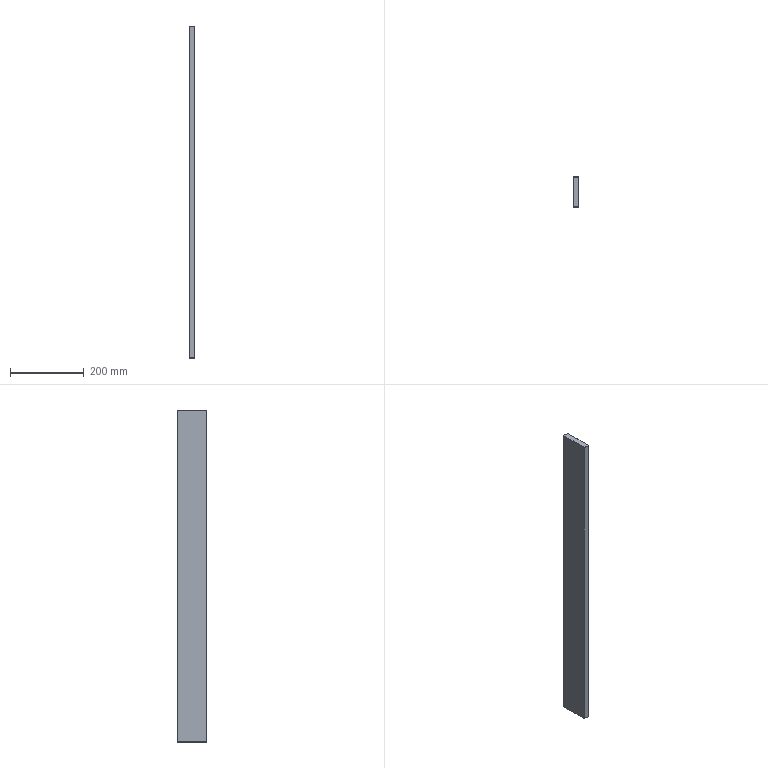Part | STEP file | HJDX-007 | 1 solid | 26 faces | box 16 x 80 x 900 mm | volume 1151503 mm3 | plane 26
STEP:
#1=CARTESIAN_POINT('',(16.,-39.5,-449.5));
#2=VERTEX_POINT('',#1);
#3=CARTESIAN_POINT('',(16.,-39.5,449.5));
#4=VERTEX_POINT('',#3);
#5=CARTESIAN_POINT('',(16.,-39.5,0.));
#6=DIRECTION('',(0.,0.,1.));
#7=VECTOR('',#6,1000.);
#8=LINE('',#5,#7);
#9=EDGE_CURVE('',#2,#4,#8,.T.);
#10=ORIENTED_EDGE('',*,*,#9,.F.);
#11=CARTESIAN_POINT('',(16.,39.5,-449.5));
#12=VERTEX_POINT('',#11);
#13=CARTESIAN_POINT('',(16.,0.,-449.5));
#14=DIRECTION('',(0.,-1.,0.));
#15=VECTOR('',#14,1000.);
#16=LINE('',#13,#15);
#17=EDGE_CURVE('',#12,#2,#16,.T.);
#18=ORIENTED_EDGE('',*,*,#17,.F.);
#19=CARTESIAN_POINT('',(16.,39.5,449.5));
#20=VERTEX_POINT('',#19);
#21=CARTESIAN_POINT('',(16.,39.5,0.));
#22=DIRECTION('',(0.,0.,-1.));
#23=VECTOR('',#22,1000.);
#24=LINE('',#21,#23);
#25=EDGE_CURVE('',#20,#12,#24,.T.);
#26=ORIENTED_EDGE('',*,*,#25,.F.);
#27=CARTESIAN_POINT('',(16.,0.,449.5));
#28=DIRECTION('',(0.,1.,0.));
#29=VECTOR('',#28,1000.);
#30=LINE('',#27,#29);
#31=EDGE_CURVE('',#4,#20,#30,.T.);
#32=ORIENTED_EDGE('',*,*,#31,.F.);
#33=EDGE_LOOP('',(#10,#18,#26,#32));
#34=FACE_OUTER_BOUND('',#33,.T.);
#35=CARTESIAN_POINT('',(16.,0.,0.));
#36=DIRECTION('',(-1.,0.,0.));
#37=DIRECTION('',(0.,0.,1.));
#38=AXIS2_PLACEMENT_3D('',#35,#36,#37);
#39=PLANE('',#38);
#40=ADVANCED_FACE('',(#34),#39,.F.);
#41=ORIENTED_EDGE('',*,*,#31,.T.);
#42=CARTESIAN_POINT('',(15.5,39.5,450.));
#43=VERTEX_POINT('',#42);
#44=CARTESIAN_POINT('',(16.,39.5,449.5));
#45=DIRECTION('',(0.7071,0.,-0.7071));
#46=VECTOR('',#45,1000.);
#47=LINE('',#44,#46);
#48=EDGE_CURVE('',#43,#20,#47,.T.);
#49=ORIENTED_EDGE('',*,*,#48,.F.);
#50=CARTESIAN_POINT('',(15.5,-39.5,450.));
#51=VERTEX_POINT('',#50);
#52=CARTESIAN_POINT('',(15.5,0.,450.));
#53=DIRECTION('',(0.,1.,0.));
#54=VECTOR('',#53,1000.);
#55=LINE('',#52,#54);
#56=EDGE_CURVE('',#51,#43,#55,.T.);
#57=ORIENTED_EDGE('',*,*,#56,.F.);
#58=CARTESIAN_POINT('',(16.,-39.5,449.5));
#59=DIRECTION('',(-0.7071,0.,0.7071));
#60=VECTOR('',#59,1000.);
#61=LINE('',#58,#60);
#62=EDGE_CURVE('',#4,#51,#61,.T.);
#63=ORIENTED_EDGE('',*,*,#62,.F.);
#64=EDGE_LOOP('',(#41,#49,#57,#63));
#65=FACE_OUTER_BOUND('',#64,.T.);
#66=CARTESIAN_POINT('',(16.,0.,449.5));
#67=DIRECTION('',(-0.7071,0.,-0.7071));
#68=DIRECTION('',(-0.7071,0.,0.7071));
#69=AXIS2_PLACEMENT_3D('',#66,#67,#68);
#70=PLANE('',#69);
#71=ADVANCED_FACE('',(#65),#70,.F.);
#72=ORIENTED_EDGE('',*,*,#9,.T.);
#73=CARTESIAN_POINT('',(15.5,-40.,449.5));
#74=VERTEX_POINT('',#73);
#75=CARTESIAN_POINT('',(16.,-39.5,449.5));
#76=DIRECTION('',(0.7071,0.7071,0.));
#77=VECTOR('',#76,1000.);
#78=LINE('',#75,#77);
#79=EDGE_CURVE('',#74,#4,#78,.T.);
#80=ORIENTED_EDGE('',*,*,#79,.F.);
#81=CARTESIAN_POINT('',(15.5,-40.,-449.5));
#82=VERTEX_POINT('',#81);
#83=CARTESIAN_POINT('',(15.5,-40.,0.));
#84=DIRECTION('',(0.,0.,1.));
#85=VECTOR('',#84,1000.);
#86=LINE('',#83,#85);
#87=EDGE_CURVE('',#82,#74,#86,.T.);
#88=ORIENTED_EDGE('',*,*,#87,.F.);
#89=CARTESIAN_POINT('',(16.,-39.5,-449.5));
#90=DIRECTION('',(-0.7071,-0.7071,0.));
#91=VECTOR('',#90,1000.);
#92=LINE('',#89,#91);
#93=EDGE_CURVE('',#2,#82,#92,.T.);
#94=ORIENTED_EDGE('',*,*,#93,.F.);
#95=EDGE_LOOP('',(#72,#80,#88,#94));
#96=FACE_OUTER_BOUND('',#95,.T.);
#97=CARTESIAN_POINT('',(16.,-39.5,0.));
#98=DIRECTION('',(-0.7071,0.7071,0.));
#99=DIRECTION('',(-0.7071,-0.7071,0.));
#100=AXIS2_PLACEMENT_3D('',#97,#98,#99);
#101=PLANE('',#100);
#102=ADVANCED_FACE('',(#96),#101,.F.);
#103=CARTESIAN_POINT('',(15.5,39.5,-450.));
#104=VERTEX_POINT('',#103);
#105=CARTESIAN_POINT('',(15.5,-39.5,-450.));
#106=VERTEX_POINT('',#105);
#107=CARTESIAN_POINT('',(15.5,0.,-450.));
#108=DIRECTION('',(0.,-1.,0.));
#109=VECTOR('',#108,1000.);
#110=LINE('',#107,#109);
#111=EDGE_CURVE('',#104,#106,#110,.T.);
#112=ORIENTED_EDGE('',*,*,#111,.F.);
#113=CARTESIAN_POINT('',(16.,39.5,-449.5));
#114=DIRECTION('',(-0.7071,0.,-0.7071));
#115=VECTOR('',#114,1000.);
#116=LINE('',#113,#115);
#117=EDGE_CURVE('',#12,#104,#116,.T.);
#118=ORIENTED_EDGE('',*,*,#117,.F.);
#119=ORIENTED_EDGE('',*,*,#17,.T.);
#120=CARTESIAN_POINT('',(16.,-39.5,-449.5));
#121=DIRECTION('',(0.7071,0.,0.7071));
#122=VECTOR('',#121,1000.);
#123=LINE('',#120,#122);
#124=EDGE_CURVE('',#106,#2,#123,.T.);
#125=ORIENTED_EDGE('',*,*,#124,.F.);
#126=EDGE_LOOP('',(#112,#118,#119,#125));
#127=FACE_OUTER_BOUND('',#126,.T.);
#128=CARTESIAN_POINT('',(16.,0.,-449.5));
#129=DIRECTION('',(-0.7071,0.,0.7071));
#130=DIRECTION('',(0.7071,0.,0.7071));
#131=AXIS2_PLACEMENT_3D('',#128,#129,#130);
#132=PLANE('',#131);
#133=ADVANCED_FACE('',(#127),#132,.F.);
#134=ORIENTED_EDGE('',*,*,#25,.T.);
#135=CARTESIAN_POINT('',(15.5,40.,-449.5));
#136=VERTEX_POINT('',#135);
#137=CARTESIAN_POINT('',(16.,39.5,-449.5));
#138=DIRECTION('',(0.7071,-0.7071,0.));
#139=VECTOR('',#138,1000.);
#140=LINE('',#137,#139);
#141=EDGE_CURVE('',#136,#12,#140,.T.);
#142=ORIENTED_EDGE('',*,*,#141,.F.);
#143=CARTESIAN_POINT('',(15.5,40.,449.5));
#144=VERTEX_POINT('',#143);
#145=CARTESIAN_POINT('',(15.5,40.,0.));
#146=DIRECTION('',(0.,0.,-1.));
#147=VECTOR('',#146,1000.);
#148=LINE('',#145,#147);
#149=EDGE_CURVE('',#144,#136,#148,.T.);
#150=ORIENTED_EDGE('',*,*,#149,.F.);
#151=CARTESIAN_POINT('',(16.,39.5,449.5));
#152=DIRECTION('',(-0.7071,0.7071,0.));
#153=VECTOR('',#152,1000.);
#154=LINE('',#151,#153);
#155=EDGE_CURVE('',#20,#144,#154,.T.);
#156=ORIENTED_EDGE('',*,*,#155,.F.);
#157=EDGE_LOOP('',(#134,#142,#150,#156));
#158=FACE_OUTER_BOUND('',#157,.T.);
#159=CARTESIAN_POINT('',(16.,39.5,0.));
#160=DIRECTION('',(-0.7071,-0.7071,0.));
#161=DIRECTION('',(0.7071,-0.7071,0.));
#162=AXIS2_PLACEMENT_3D('',#159,#160,#161);
#163=PLANE('',#162);
#164=ADVANCED_FACE('',(#158),#163,.F.);
#165=ORIENTED_EDGE('',*,*,#79,.T.);
#166=ORIENTED_EDGE('',*,*,#62,.T.);
#167=CARTESIAN_POINT('',(15.5,-40.,449.5));
#168=DIRECTION('',(0.,-0.7071,-0.7071));
#169=VECTOR('',#168,1000.);
#170=LINE('',#167,#169);
#171=EDGE_CURVE('',#51,#74,#170,.T.);
#172=ORIENTED_EDGE('',*,*,#171,.T.);
#173=EDGE_LOOP('',(#165,#166,#172));
#174=FACE_OUTER_BOUND('',#173,.T.);
#175=CARTESIAN_POINT('',(15.5,-39.5,450.));
#176=DIRECTION('',(0.5774,-0.5774,0.5774));
#177=DIRECTION('',(0.7071,0.,-0.7071));
#178=AXIS2_PLACEMENT_3D('',#175,#176,#177);
#179=PLANE('',#178);
#180=ADVANCED_FACE('',(#174),#179,.T.);
#181=ORIENTED_EDGE('',*,*,#155,.T.);
#182=CARTESIAN_POINT('',(15.5,39.5,450.));
#183=DIRECTION('',(0.,-0.7071,0.7071));
#184=VECTOR('',#183,1000.);
#185=LINE('',#182,#184);
#186=EDGE_CURVE('',#144,#43,#185,.T.);
#187=ORIENTED_EDGE('',*,*,#186,.T.);
#188=ORIENTED_EDGE('',*,*,#48,.T.);
#189=EDGE_LOOP('',(#181,#187,#188));
#190=FACE_OUTER_BOUND('',#189,.T.);
#191=CARTESIAN_POINT('',(15.5,40.,449.5));
#192=DIRECTION('',(0.5774,0.5774,0.5774));
#193=DIRECTION('',(0.7071,0.,-0.7071));
#194=AXIS2_PLACEMENT_3D('',#191,#192,#193);
#195=PLANE('',#194);
#196=ADVANCED_FACE('',(#190),#195,.T.);
#197=CARTESIAN_POINT('',(0.5,39.5,450.));
#198=VERTEX_POINT('',#197);
#199=CARTESIAN_POINT('',(16.,39.5,450.));
#200=DIRECTION('',(1.,0.,0.));
#201=VECTOR('',#200,1000.);
#202=LINE('',#199,#201);
#203=EDGE_CURVE('',#198,#43,#202,.T.);
#204=ORIENTED_EDGE('',*,*,#203,.F.);
#205=CARTESIAN_POINT('',(0.5,-39.5,450.));
#206=VERTEX_POINT('',#205);
#207=CARTESIAN_POINT('',(0.5,-40.,450.));
#208=DIRECTION('',(0.,1.,0.));
#209=VECTOR('',#208,1000.);
#210=LINE('',#207,#209);
#211=EDGE_CURVE('',#206,#198,#210,.T.);
#212=ORIENTED_EDGE('',*,*,#211,.F.);
#213=CARTESIAN_POINT('',(16.,-39.5,450.));
#214=DIRECTION('',(-1.,0.,0.));
#215=VECTOR('',#214,1000.);
#216=LINE('',#213,#215);
#217=EDGE_CURVE('',#51,#206,#216,.T.);
#218=ORIENTED_EDGE('',*,*,#217,.F.);
#219=ORIENTED_EDGE('',*,*,#56,.T.);
#220=EDGE_LOOP('',(#204,#212,#218,#219));
#221=FACE_OUTER_BOUND('',#220,.T.);
#222=CARTESIAN_POINT('',(16.,-40.,450.));
#223=DIRECTION('',(0.,0.,-1.));
#224=DIRECTION('',(-1.,0.,0.));
#225=AXIS2_PLACEMENT_3D('',#222,#223,#224);
#226=PLANE('',#225);
#227=ADVANCED_FACE('',(#221),#226,.F.);
#228=ORIENTED_EDGE('',*,*,#93,.T.);
#229=CARTESIAN_POINT('',(15.5,-39.5,-450.));
#230=DIRECTION('',(0.,0.7071,-0.7071));
#231=VECTOR('',#230,1000.);
#232=LINE('',#229,#231);
#233=EDGE_CURVE('',#82,#106,#232,.T.);
#234=ORIENTED_EDGE('',*,*,#233,.T.);
#235=ORIENTED_EDGE('',*,*,#124,.T.);
#236=EDGE_LOOP('',(#228,#234,#235));
#237=FACE_OUTER_BOUND('',#236,.T.);
#238=CARTESIAN_POINT('',(16.,-39.5,-449.5));
#239=DIRECTION('',(0.5774,-0.5774,-0.5774));
#240=DIRECTION('',(-0.7071,0.,-0.7071));
#241=AXIS2_PLACEMENT_3D('',#238,#239,#240);
#242=PLANE('',#241);
#243=ADVANCED_FACE('',(#237),#242,.T.);
#244=CARTESIAN_POINT('',(0.5,-40.,-449.5));
#245=VERTEX_POINT('',#244);
#246=CARTESIAN_POINT('',(0.5,-40.,449.5));
#247=VERTEX_POINT('',#246);
#248=CARTESIAN_POINT('',(0.5,-40.,450.));
#249=DIRECTION('',(0.,0.,1.));
#250=VECTOR('',#249,1000.);
#251=LINE('',#248,#250);
#252=EDGE_CURVE('',#245,#247,#251,.T.);
#253=ORIENTED_EDGE('',*,*,#252,.F.);
#254=CARTESIAN_POINT('',(16.,-40.,-449.5));
#255=DIRECTION('',(-1.,0.,0.));
#256=VECTOR('',#255,1000.);
#257=LINE('',#254,#256);
#258=EDGE_CURVE('',#82,#245,#257,.T.);
#259=ORIENTED_EDGE('',*,*,#258,.F.);
#260=ORIENTED_EDGE('',*,*,#87,.T.);
#261=CARTESIAN_POINT('',(16.,-40.,449.5));
#262=DIRECTION('',(1.,0.,0.));
#263=VECTOR('',#262,1000.);
#264=LINE('',#261,#263);
#265=EDGE_CURVE('',#247,#74,#264,.T.);
#266=ORIENTED_EDGE('',*,*,#265,.F.);
#267=EDGE_LOOP('',(#253,#259,#260,#266));
#268=FACE_OUTER_BOUND('',#267,.T.);
#269=CARTESIAN_POINT('',(16.,-40.,450.));
#270=DIRECTION('',(0.,1.,0.));
#271=DIRECTION('',(0.,0.,1.));
#272=AXIS2_PLACEMENT_3D('',#269,#270,#271);
#273=PLANE('',#272);
#274=ADVANCED_FACE('',(#268),#273,.F.);
#275=CARTESIAN_POINT('',(0.5,-39.5,-450.));
#276=VERTEX_POINT('',#275);
#277=CARTESIAN_POINT('',(16.,-39.5,-450.));
#278=DIRECTION('',(1.,0.,0.));
#279=VECTOR('',#278,1000.);
#280=LINE('',#277,#279);
#281=EDGE_CURVE('',#276,#106,#280,.T.);
#282=ORIENTED_EDGE('',*,*,#281,.F.);
#283=CARTESIAN_POINT('',(0.5,39.5,-450.));
#284=VERTEX_POINT('',#283);
#285=CARTESIAN_POINT('',(0.5,-40.,-450.));
#286=DIRECTION('',(0.,-1.,0.));
#287=VECTOR('',#286,1000.);
#288=LINE('',#285,#287);
#289=EDGE_CURVE('',#284,#276,#288,.T.);
#290=ORIENTED_EDGE('',*,*,#289,.F.);
#291=CARTESIAN_POINT('',(16.,39.5,-450.));
#292=DIRECTION('',(-1.,0.,0.));
#293=VECTOR('',#292,1000.);
#294=LINE('',#291,#293);
#295=EDGE_CURVE('',#104,#284,#294,.T.);
#296=ORIENTED_EDGE('',*,*,#295,.F.);
#297=ORIENTED_EDGE('',*,*,#111,.T.);
#298=EDGE_LOOP('',(#282,#290,#296,#297));
#299=FACE_OUTER_BOUND('',#298,.T.);
#300=CARTESIAN_POINT('',(16.,-40.,-450.));
#301=DIRECTION('',(0.,0.,1.));
#302=DIRECTION('',(1.,0.,0.));
#303=AXIS2_PLACEMENT_3D('',#300,#301,#302);
#304=PLANE('',#303);
#305=ADVANCED_FACE('',(#299),#304,.F.);
#306=ORIENTED_EDGE('',*,*,#117,.T.);
#307=CARTESIAN_POINT('',(15.5,39.5,-450.));
#308=DIRECTION('',(0.,0.7071,0.7071));
#309=VECTOR('',#308,1000.);
#310=LINE('',#307,#309);
#311=EDGE_CURVE('',#104,#136,#310,.T.);
#312=ORIENTED_EDGE('',*,*,#311,.T.);
#313=ORIENTED_EDGE('',*,*,#141,.T.);
#314=EDGE_LOOP('',(#306,#312,#313));
#315=FACE_OUTER_BOUND('',#314,.T.);
#316=CARTESIAN_POINT('',(15.5,40.,-449.5));
#317=DIRECTION('',(0.5774,0.5774,-0.5774));
#318=DIRECTION('',(-0.7071,0.,-0.7071));
#319=AXIS2_PLACEMENT_3D('',#316,#317,#318);
#320=PLANE('',#319);
#321=ADVANCED_FACE('',(#315),#320,.T.);
#322=CARTESIAN_POINT('',(0.5,40.,449.5));
#323=VERTEX_POINT('',#322);
#324=CARTESIAN_POINT('',(0.5,40.,-449.5));
#325=VERTEX_POINT('',#324);
#326=CARTESIAN_POINT('',(0.5,40.,450.));
#327=DIRECTION('',(0.,0.,-1.));
#328=VECTOR('',#327,1000.);
#329=LINE('',#326,#328);
#330=EDGE_CURVE('',#323,#325,#329,.T.);
#331=ORIENTED_EDGE('',*,*,#330,.F.);
#332=CARTESIAN_POINT('',(16.,40.,449.5));
#333=DIRECTION('',(-1.,0.,0.));
#334=VECTOR('',#333,1000.);
#335=LINE('',#332,#334);
#336=EDGE_CURVE('',#144,#323,#335,.T.);
#337=ORIENTED_EDGE('',*,*,#336,.F.);
#338=ORIENTED_EDGE('',*,*,#149,.T.);
#339=CARTESIAN_POINT('',(16.,40.,-449.5));
#340=DIRECTION('',(1.,0.,0.));
#341=VECTOR('',#340,1000.);
#342=LINE('',#339,#341);
#343=EDGE_CURVE('',#325,#136,#342,.T.);
#344=ORIENTED_EDGE('',*,*,#343,.F.);
#345=EDGE_LOOP('',(#331,#337,#338,#344));
#346=FACE_OUTER_BOUND('',#345,.T.);
#347=CARTESIAN_POINT('',(16.,40.,450.));
#348=DIRECTION('',(0.,-1.,0.));
#349=DIRECTION('',(0.,0.,-1.));
#350=AXIS2_PLACEMENT_3D('',#347,#348,#349);
#351=PLANE('',#350);
#352=ADVANCED_FACE('',(#346),#351,.F.);
#353=ORIENTED_EDGE('',*,*,#336,.T.);
#354=CARTESIAN_POINT('',(0.5,39.5,450.));
#355=DIRECTION('',(0.,0.7071,-0.7071));
#356=VECTOR('',#355,1000.);
#357=LINE('',#354,#356);
#358=EDGE_CURVE('',#198,#323,#357,.T.);
#359=ORIENTED_EDGE('',*,*,#358,.F.);
#360=ORIENTED_EDGE('',*,*,#203,.T.);
#361=ORIENTED_EDGE('',*,*,#186,.F.);
#362=EDGE_LOOP('',(#353,#359,#360,#361));
#363=FACE_OUTER_BOUND('',#362,.T.);
#364=CARTESIAN_POINT('',(16.,39.5,450.));
#365=DIRECTION('',(0.,-0.7071,-0.7071));
#366=DIRECTION('',(0.,0.7071,-0.7071));
#367=AXIS2_PLACEMENT_3D('',#364,#365,#366);
#368=PLANE('',#367);
#369=ADVANCED_FACE('',(#363),#368,.F.);
#370=CARTESIAN_POINT('',(0.,39.5,449.5));
#371=VERTEX_POINT('',#370);
#372=CARTESIAN_POINT('',(0.5,39.5,450.));
#373=DIRECTION('',(-0.7071,0.,-0.7071));
#374=VECTOR('',#373,1000.);
#375=LINE('',#372,#374);
#376=EDGE_CURVE('',#198,#371,#375,.T.);
#377=ORIENTED_EDGE('',*,*,#376,.T.);
#378=CARTESIAN_POINT('',(0.,-39.5,449.5));
#379=VERTEX_POINT('',#378);
#380=CARTESIAN_POINT('',(0.,-40.,449.5));
#381=DIRECTION('',(0.,-1.,0.));
#382=VECTOR('',#381,1000.);
#383=LINE('',#380,#382);
#384=EDGE_CURVE('',#371,#379,#383,.T.);
#385=ORIENTED_EDGE('',*,*,#384,.T.);
#386=CARTESIAN_POINT('',(0.5,-39.5,450.));
#387=DIRECTION('',(0.7071,0.,0.7071));
#388=VECTOR('',#387,1000.);
#389=LINE('',#386,#388);
#390=EDGE_CURVE('',#379,#206,#389,.T.);
#391=ORIENTED_EDGE('',*,*,#390,.T.);
#392=ORIENTED_EDGE('',*,*,#211,.T.);
#393=EDGE_LOOP('',(#377,#385,#391,#392));
#394=FACE_OUTER_BOUND('',#393,.T.);
#395=CARTESIAN_POINT('',(0.5,-40.,450.));
#396=DIRECTION('',(-0.7071,0.,0.7071));
#397=DIRECTION('',(0.7071,0.,0.7071));
#398=AXIS2_PLACEMENT_3D('',#395,#396,#397);
#399=PLANE('',#398);
#400=ADVANCED_FACE('',(#394),#399,.T.);
#401=ORIENTED_EDGE('',*,*,#217,.T.);
#402=CARTESIAN_POINT('',(0.5,-40.,449.5));
#403=DIRECTION('',(0.,0.7071,0.7071));
#404=VECTOR('',#403,1000.);
#405=LINE('',#402,#404);
#406=EDGE_CURVE('',#247,#206,#405,.T.);
#407=ORIENTED_EDGE('',*,*,#406,.F.);
#408=ORIENTED_EDGE('',*,*,#265,.T.);
#409=ORIENTED_EDGE('',*,*,#171,.F.);
#410=EDGE_LOOP('',(#401,#407,#408,#409));
#411=FACE_OUTER_BOUND('',#410,.T.);
#412=CARTESIAN_POINT('',(16.,-40.,449.5));
#413=DIRECTION('',(0.,0.7071,-0.7071));
#414=DIRECTION('',(0.,0.7071,0.7071));
#415=AXIS2_PLACEMENT_3D('',#412,#413,#414);
#416=PLANE('',#415);
#417=ADVANCED_FACE('',(#411),#416,.F.);
#418=CARTESIAN_POINT('',(0.5,-40.,449.5));
#419=DIRECTION('',(-0.7071,0.7071,0.));
#420=VECTOR('',#419,1000.);
#421=LINE('',#418,#420);
#422=EDGE_CURVE('',#247,#379,#421,.T.);
#423=ORIENTED_EDGE('',*,*,#422,.T.);
#424=CARTESIAN_POINT('',(0.,-39.5,-449.5));
#425=VERTEX_POINT('',#424);
#426=CARTESIAN_POINT('',(0.,-39.5,450.));
#427=DIRECTION('',(0.,0.,-1.));
#428=VECTOR('',#427,1000.);
#429=LINE('',#426,#428);
#430=EDGE_CURVE('',#379,#425,#429,.T.);
#431=ORIENTED_EDGE('',*,*,#430,.T.);
#432=CARTESIAN_POINT('',(0.5,-40.,-449.5));
#433=DIRECTION('',(0.7071,-0.7071,0.));
#434=VECTOR('',#433,1000.);
#435=LINE('',#432,#434);
#436=EDGE_CURVE('',#425,#245,#435,.T.);
#437=ORIENTED_EDGE('',*,*,#436,.T.);
#438=ORIENTED_EDGE('',*,*,#252,.T.);
#439=EDGE_LOOP('',(#423,#431,#437,#438));
#440=FACE_OUTER_BOUND('',#439,.T.);
#441=CARTESIAN_POINT('',(0.5,-40.,450.));
#442=DIRECTION('',(-0.7071,-0.7071,0.));
#443=DIRECTION('',(0.7071,-0.7071,0.));
#444=AXIS2_PLACEMENT_3D('',#441,#442,#443);
#445=PLANE('',#444);
#446=ADVANCED_FACE('',(#440),#445,.T.);
#447=ORIENTED_EDGE('',*,*,#258,.T.);
#448=CARTESIAN_POINT('',(0.5,-39.5,-450.));
#449=DIRECTION('',(0.,-0.7071,0.7071));
#450=VECTOR('',#449,1000.);
#451=LINE('',#448,#450);
#452=EDGE_CURVE('',#276,#245,#451,.T.);
#453=ORIENTED_EDGE('',*,*,#452,.F.);
#454=ORIENTED_EDGE('',*,*,#281,.T.);
#455=ORIENTED_EDGE('',*,*,#233,.F.);
#456=EDGE_LOOP('',(#447,#453,#454,#455));
#457=FACE_OUTER_BOUND('',#456,.T.);
#458=CARTESIAN_POINT('',(16.,-39.5,-450.));
#459=DIRECTION('',(0.,0.7071,0.7071));
#460=DIRECTION('',(0.,-0.7071,0.7071));
#461=AXIS2_PLACEMENT_3D('',#458,#459,#460);
#462=PLANE('',#461);
#463=ADVANCED_FACE('',(#457),#462,.F.);
#464=CARTESIAN_POINT('',(0.,39.5,-449.5));
#465=VERTEX_POINT('',#464);
#466=CARTESIAN_POINT('',(0.5,39.5,-450.));
#467=DIRECTION('',(0.7071,0.,-0.7071));
#468=VECTOR('',#467,1000.);
#469=LINE('',#466,#468);
#470=EDGE_CURVE('',#465,#284,#469,.T.);
#471=ORIENTED_EDGE('',*,*,#470,.T.);
#472=ORIENTED_EDGE('',*,*,#289,.T.);
#473=CARTESIAN_POINT('',(0.5,-39.5,-450.));
#474=DIRECTION('',(-0.7071,0.,0.7071));
#475=VECTOR('',#474,1000.);
#476=LINE('',#473,#475);
#477=EDGE_CURVE('',#276,#425,#476,.T.);
#478=ORIENTED_EDGE('',*,*,#477,.T.);
#479=CARTESIAN_POINT('',(0.,-40.,-449.5));
#480=DIRECTION('',(0.,1.,0.));
#481=VECTOR('',#480,1000.);
#482=LINE('',#479,#481);
#483=EDGE_CURVE('',#425,#465,#482,.T.);
#484=ORIENTED_EDGE('',*,*,#483,.T.);
#485=EDGE_LOOP('',(#471,#472,#478,#484));
#486=FACE_OUTER_BOUND('',#485,.T.);
#487=CARTESIAN_POINT('',(0.5,-40.,-450.));
#488=DIRECTION('',(-0.7071,0.,-0.7071));
#489=DIRECTION('',(-0.7071,0.,0.7071));
#490=AXIS2_PLACEMENT_3D('',#487,#488,#489);
#491=PLANE('',#490);
#492=ADVANCED_FACE('',(#486),#491,.T.);
#493=ORIENTED_EDGE('',*,*,#295,.T.);
#494=CARTESIAN_POINT('',(0.5,40.,-449.5));
#495=DIRECTION('',(0.,-0.7071,-0.7071));
#496=VECTOR('',#495,1000.);
#497=LINE('',#494,#496);
#498=EDGE_CURVE('',#325,#284,#497,.T.);
#499=ORIENTED_EDGE('',*,*,#498,.F.);
#500=ORIENTED_EDGE('',*,*,#343,.T.);
#501=ORIENTED_EDGE('',*,*,#311,.F.);
#502=EDGE_LOOP('',(#493,#499,#500,#501));
#503=FACE_OUTER_BOUND('',#502,.T.);
#504=CARTESIAN_POINT('',(16.,40.,-449.5));
#505=DIRECTION('',(0.,-0.7071,0.7071));
#506=DIRECTION('',(0.,-0.7071,-0.7071));
#507=AXIS2_PLACEMENT_3D('',#504,#505,#506);
#508=PLANE('',#507);
#509=ADVANCED_FACE('',(#503),#508,.F.);
#510=CARTESIAN_POINT('',(0.5,40.,449.5));
#511=DIRECTION('',(0.7071,0.7071,0.));
#512=VECTOR('',#511,1000.);
#513=LINE('',#510,#512);
#514=EDGE_CURVE('',#371,#323,#513,.T.);
#515=ORIENTED_EDGE('',*,*,#514,.T.);
#516=ORIENTED_EDGE('',*,*,#330,.T.);
#517=CARTESIAN_POINT('',(0.5,40.,-449.5));
#518=DIRECTION('',(-0.7071,-0.7071,0.));
#519=VECTOR('',#518,1000.);
#520=LINE('',#517,#519);
#521=EDGE_CURVE('',#325,#465,#520,.T.);
#522=ORIENTED_EDGE('',*,*,#521,.T.);
#523=CARTESIAN_POINT('',(0.,39.5,450.));
#524=DIRECTION('',(0.,0.,1.));
#525=VECTOR('',#524,1000.);
#526=LINE('',#523,#525);
#527=EDGE_CURVE('',#465,#371,#526,.T.);
#528=ORIENTED_EDGE('',*,*,#527,.T.);
#529=EDGE_LOOP('',(#515,#516,#522,#528));
#530=FACE_OUTER_BOUND('',#529,.T.);
#531=CARTESIAN_POINT('',(0.5,40.,450.));
#532=DIRECTION('',(-0.7071,0.7071,0.));
#533=DIRECTION('',(-0.7071,-0.7071,0.));
#534=AXIS2_PLACEMENT_3D('',#531,#532,#533);
#535=PLANE('',#534);
#536=ADVANCED_FACE('',(#530),#535,.T.);
#537=ORIENTED_EDGE('',*,*,#358,.T.);
#538=ORIENTED_EDGE('',*,*,#514,.F.);
#539=ORIENTED_EDGE('',*,*,#376,.F.);
#540=EDGE_LOOP('',(#537,#538,#539));
#541=FACE_OUTER_BOUND('',#540,.T.);
#542=CARTESIAN_POINT('',(0.5,40.,449.5));
#543=DIRECTION('',(-0.5774,0.5774,0.5774));
#544=DIRECTION('',(0.7071,0.,0.7071));
#545=AXIS2_PLACEMENT_3D('',#542,#543,#544);
#546=PLANE('',#545);
#547=ADVANCED_FACE('',(#541),#546,.T.);
#548=ORIENTED_EDGE('',*,*,#527,.F.);
#549=ORIENTED_EDGE('',*,*,#483,.F.);
#550=ORIENTED_EDGE('',*,*,#430,.F.);
#551=ORIENTED_EDGE('',*,*,#384,.F.);
#552=EDGE_LOOP('',(#548,#549,#550,#551));
#553=FACE_OUTER_BOUND('',#552,.T.);
#554=CARTESIAN_POINT('',(0.,0.,0.));
#555=DIRECTION('',(-1.,0.,0.));
#556=DIRECTION('',(0.,0.,1.));
#557=AXIS2_PLACEMENT_3D('',#554,#555,#556);
#558=PLANE('',#557);
#559=ADVANCED_FACE('',(#553),#558,.T.);
#560=ORIENTED_EDGE('',*,*,#406,.T.);
#561=ORIENTED_EDGE('',*,*,#390,.F.);
#562=ORIENTED_EDGE('',*,*,#422,.F.);
#563=EDGE_LOOP('',(#560,#561,#562));
#564=FACE_OUTER_BOUND('',#563,.T.);
#565=CARTESIAN_POINT('',(0.,-39.5,449.5));
#566=DIRECTION('',(-0.5774,-0.5774,0.5774));
#567=DIRECTION('',(0.7071,0.,0.7071));
#568=AXIS2_PLACEMENT_3D('',#565,#566,#567);
#569=PLANE('',#568);
#570=ADVANCED_FACE('',(#564),#569,.T.);
#571=ORIENTED_EDGE('',*,*,#436,.F.);
#572=ORIENTED_EDGE('',*,*,#477,.F.);
#573=ORIENTED_EDGE('',*,*,#452,.T.);
#574=EDGE_LOOP('',(#571,#572,#573));
#575=FACE_OUTER_BOUND('',#574,.T.);
#576=CARTESIAN_POINT('',(0.5,-40.,-449.5));
#577=DIRECTION('',(-0.5774,-0.5774,-0.5774));
#578=DIRECTION('',(-0.7071,0.,0.7071));
#579=AXIS2_PLACEMENT_3D('',#576,#577,#578);
#580=PLANE('',#579);
#581=ADVANCED_FACE('',(#575),#580,.T.);
#582=ORIENTED_EDGE('',*,*,#470,.F.);
#583=ORIENTED_EDGE('',*,*,#521,.F.);
#584=ORIENTED_EDGE('',*,*,#498,.T.);
#585=EDGE_LOOP('',(#582,#583,#584));
#586=FACE_OUTER_BOUND('',#585,.T.);
#587=CARTESIAN_POINT('',(0.,39.5,-449.5));
#588=DIRECTION('',(-0.5774,0.5774,-0.5774));
#589=DIRECTION('',(-0.7071,0.,0.7071));
#590=AXIS2_PLACEMENT_3D('',#587,#588,#589);
#591=PLANE('',#590);
#592=ADVANCED_FACE('',(#586),#591,.T.);
#593=CLOSED_SHELL('',(#40,#71,#102,#133,#164,#180,#196,#227,#243,#274,#305,#321,#352,#369,#400,#417,#446,#463,#492,#509,#536,#547,#559,#570,#581,#592));
#594=MANIFOLD_SOLID_BREP('',#593);
#595=CARTESIAN_POINT('',(0.,0.,0.));
#596=DIRECTION('',(0.,0.,1.));
#597=DIRECTION('',(1.,0.,0.));
#598=AXIS2_PLACEMENT_3D('',#595,#596,#597);
#599=(LENGTH_UNIT()NAMED_UNIT(*)SI_UNIT(.MILLI.,.METRE.));
#600=UNCERTAINTY_MEASURE_WITH_UNIT(LENGTH_MEASURE(0.00001),#599,'','');
#601=(NAMED_UNIT(*)PLANE_ANGLE_UNIT()SI_UNIT($,.RADIAN.));
#602=(NAMED_UNIT(*)SI_UNIT($,.STERADIAN.)SOLID_ANGLE_UNIT());
#603=(GEOMETRIC_REPRESENTATION_CONTEXT(3)GLOBAL_UNCERTAINTY_ASSIGNED_CONTEXT((#600))GLOBAL_UNIT_ASSIGNED_CONTEXT((#599,#601,#602))REPRESENTATION_CONTEXT('',''));
#604=ADVANCED_BREP_SHAPE_REPRESENTATION('',(#594,#598),#603);